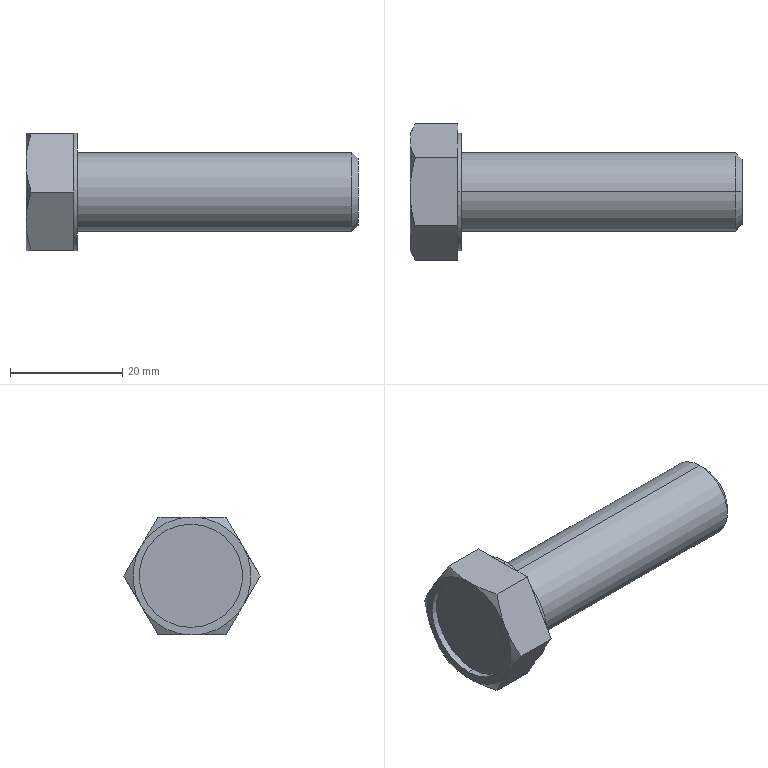Part | STEP file | formed hex screw_am_B18.2.3.2M - Formed hex screw, M14 x 2.0 x 50 --34WN | 1 solid | 30 faces | box 59.09 x 24.249 x 21 mm | volume 10811 mm3 | plane 16 | cone 8 | cylinder 6 | commonest cylinder face diameters 14 x2 18.375 x2 21 x2